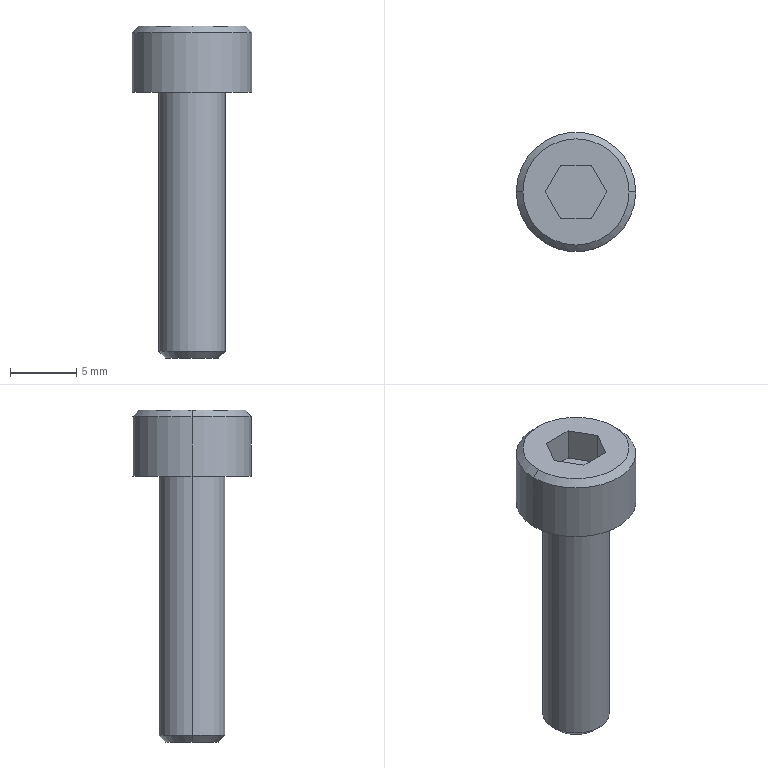Part | STEP file | _GAY01-D20-003_2.stp | 1 solid | 18 faces | box 9 x 9 x 25 mm | volume 670.975 mm3 | plane 10 | cone 4 | cylinder 4 | commonest cylinder face diameters 5 x2 9 x2
STEP:
#1=CARTESIAN_POINT('',(0.,0.,0.));
#2=DIRECTION('',(0.,0.,1.));
#3=DIRECTION('',(1.,0.,0.));
#4=AXIS2_PLACEMENT_3D('',#1,#2,#3);
#5=CARTESIAN_POINT('',(-2.01,0.,-20.));
#6=VERTEX_POINT('',#5);
#7=CARTESIAN_POINT('',(2.01,0.,-20.));
#8=VERTEX_POINT('',#7);
#9=CARTESIAN_POINT('',(0.,0.,-20.));
#10=DIRECTION('',(0.,0.,-1.));
#11=DIRECTION('',(-1.,0.,0.));
#12=AXIS2_PLACEMENT_3D('',#9,#10,#11);
#13=CIRCLE('',#12,2.01);
#14=CARTESIAN_POINT('',(0.,0.,-19.509));
#15=DIRECTION('',(0.,0.,1.));
#16=DIRECTION('',(1.,0.,0.));
#17=AXIS2_PLACEMENT_3D('',#14,#15,#16);
#18=CONICAL_SURFACE('',#17,2.5,0.7854);
#19=CARTESIAN_POINT('',(3.142,-0.4905));
#20=DIRECTION('',(-1.,0.));
#21=VECTOR('',#20,1.);
#22=LINE('',#19,#21);
#23=(GEOMETRIC_REPRESENTATION_CONTEXT(2)PARAMETRIC_REPRESENTATION_CONTEXT()REPRESENTATION_CONTEXT('',''));
#24=DEFINITIONAL_REPRESENTATION('',(#22),#23);
#25=PCURVE('',#18,#24);
#26=CARTESIAN_POINT('',(0.,2.01,-20.));
#27=DIRECTION('',(0.,0.,1.));
#28=DIRECTION('',(1.,0.,0.));
#29=AXIS2_PLACEMENT_3D('',#26,#27,#28);
#30=PLANE('',#29);
#31=CARTESIAN_POINT('',(-2.01,-2.01));
#32=CARTESIAN_POINT('',(-2.01,1.471));
#33=CARTESIAN_POINT('',(1.005,-0.2692));
#34=CARTESIAN_POINT('',(4.019,-2.01));
#35=CARTESIAN_POINT('',(1.005,-3.75));
#36=CARTESIAN_POINT('',(-2.01,-5.49));
#37=CARTESIAN_POINT('',(-2.01,-2.01));
#38=(BOUNDED_CURVE()B_SPLINE_CURVE(2,(#31,#32,#33,#34,#35,#36,#37),.UNSPECIFIED.,.T.,.F.)B_SPLINE_CURVE_WITH_KNOTS((1,2,2,2,2,1),(-2.094,0.,2.094,4.189,6.283,8.378),.UNSPECIFIED.)CURVE()GEOMETRIC_REPRESENTATION_ITEM()RATIONAL_B_SPLINE_CURVE((1.,0.5,1.,0.5,1.,0.5,1.))REPRESENTATION_ITEM(''));
#39=(GEOMETRIC_REPRESENTATION_CONTEXT(2)PARAMETRIC_REPRESENTATION_CONTEXT()REPRESENTATION_CONTEXT('',''));
#40=DEFINITIONAL_REPRESENTATION('',(#38),#39);
#41=PCURVE('',#30,#40);
#42=SURFACE_CURVE('',#13,(#25,#41),.PCURVE_S1.);
#43=EDGE_CURVE('',#6,#8,#42,.T.);
#44=ORIENTED_EDGE('',*,*,#43,.F.);
#45=CARTESIAN_POINT('',(-2.5,0.,-19.509));
#46=VERTEX_POINT('',#45);
#47=CARTESIAN_POINT('',(-2.5,0.,-19.509));
#48=DIRECTION('',(-0.7071,0.,0.7071));
#49=VECTOR('',#48,1.);
#50=LINE('',#47,#49);
#51=CARTESIAN_POINT('',(3.142,0.));
#52=DIRECTION('',(0.,1.));
#53=VECTOR('',#52,1.);
#54=LINE('',#51,#53);
#55=(GEOMETRIC_REPRESENTATION_CONTEXT(2)PARAMETRIC_REPRESENTATION_CONTEXT()REPRESENTATION_CONTEXT('',''));
#56=DEFINITIONAL_REPRESENTATION('',(#54),#55);
#57=PCURVE('',#18,#56);
#58=CARTESIAN_POINT('',(0.,0.,-19.509));
#59=DIRECTION('',(0.,0.,1.));
#60=DIRECTION('',(1.,0.,0.));
#61=AXIS2_PLACEMENT_3D('',#58,#59,#60);
#62=CONICAL_SURFACE('',#61,2.5,0.7854);
#63=CARTESIAN_POINT('',(3.142,0.));
#64=DIRECTION('',(0.,1.));
#65=VECTOR('',#64,1.);
#66=LINE('',#63,#65);
#67=(GEOMETRIC_REPRESENTATION_CONTEXT(2)PARAMETRIC_REPRESENTATION_CONTEXT()REPRESENTATION_CONTEXT('',''));
#68=DEFINITIONAL_REPRESENTATION('',(#66),#67);
#69=PCURVE('',#62,#68);
#70=SURFACE_CURVE('',#50,(#57,#69),.PCURVE_S1.);
#71=EDGE_CURVE('',#6,#46,#70,.T.);
#72=ORIENTED_EDGE('',*,*,#71,.T.);
#73=CARTESIAN_POINT('',(2.5,0.,-19.509));
#74=VERTEX_POINT('',#73);
#75=CARTESIAN_POINT('',(0.,0.,-19.509));
#76=DIRECTION('',(0.,0.,-1.));
#77=DIRECTION('',(-1.,0.,0.));
#78=AXIS2_PLACEMENT_3D('',#75,#76,#77);
#79=CIRCLE('',#78,2.5);
#80=CARTESIAN_POINT('',(3.142,0.));
#81=DIRECTION('',(-1.,0.));
#82=VECTOR('',#81,1.);
#83=LINE('',#80,#82);
#84=(GEOMETRIC_REPRESENTATION_CONTEXT(2)PARAMETRIC_REPRESENTATION_CONTEXT()REPRESENTATION_CONTEXT('',''));
#85=DEFINITIONAL_REPRESENTATION('',(#83),#84);
#86=PCURVE('',#18,#85);
#87=CARTESIAN_POINT('',(0.,0.,-20.));
#88=DIRECTION('',(0.,0.,1.));
#89=DIRECTION('',(-1.,0.,0.));
#90=AXIS2_PLACEMENT_3D('',#87,#88,#89);
#91=CYLINDRICAL_SURFACE('',#90,2.5);
#92=CARTESIAN_POINT('',(6.283,0.4905));
#93=DIRECTION('',(-1.,0.));
#94=VECTOR('',#93,1.);
#95=LINE('',#92,#94);
#96=(GEOMETRIC_REPRESENTATION_CONTEXT(2)PARAMETRIC_REPRESENTATION_CONTEXT()REPRESENTATION_CONTEXT('',''));
#97=DEFINITIONAL_REPRESENTATION('',(#95),#96);
#98=PCURVE('',#91,#97);
#99=SURFACE_CURVE('',#79,(#86,#98),.PCURVE_S1.);
#100=EDGE_CURVE('',#46,#74,#99,.T.);
#101=ORIENTED_EDGE('',*,*,#100,.T.);
#102=CARTESIAN_POINT('',(2.5,0.,-19.509));
#103=DIRECTION('',(0.7071,0.,0.7071));
#104=VECTOR('',#103,1.);
#105=LINE('',#102,#104);
#106=CARTESIAN_POINT('',(0.,0.));
#107=DIRECTION('',(0.,1.));
#108=VECTOR('',#107,1.);
#109=LINE('',#106,#108);
#110=(GEOMETRIC_REPRESENTATION_CONTEXT(2)PARAMETRIC_REPRESENTATION_CONTEXT()REPRESENTATION_CONTEXT('',''));
#111=DEFINITIONAL_REPRESENTATION('',(#109),#110);
#112=PCURVE('',#18,#111);
#113=CARTESIAN_POINT('',(6.283,0.));
#114=DIRECTION('',(0.,1.));
#115=VECTOR('',#114,1.);
#116=LINE('',#113,#115);
#117=(GEOMETRIC_REPRESENTATION_CONTEXT(2)PARAMETRIC_REPRESENTATION_CONTEXT()REPRESENTATION_CONTEXT('',''));
#118=DEFINITIONAL_REPRESENTATION('',(#116),#117);
#119=PCURVE('',#62,#118);
#120=SURFACE_CURVE('',#105,(#112,#119),.PCURVE_S1.);
#121=EDGE_CURVE('',#8,#74,#120,.T.);
#122=ORIENTED_EDGE('',*,*,#121,.F.);
#123=EDGE_LOOP('',(#44,#72,#101,#122));
#124=FACE_BOUND('',#123,.T.);
#125=ADVANCED_FACE('',(#124),#18,.T.);
#126=CARTESIAN_POINT('',(0.,0.,-19.509));
#127=DIRECTION('',(0.,0.,-1.));
#128=DIRECTION('',(-1.,0.,0.));
#129=AXIS2_PLACEMENT_3D('',#126,#127,#128);
#130=CIRCLE('',#129,2.5);
#131=CARTESIAN_POINT('',(0.,0.,-20.));
#132=DIRECTION('',(0.,0.,1.));
#133=DIRECTION('',(-1.,0.,0.));
#134=AXIS2_PLACEMENT_3D('',#131,#132,#133);
#135=CYLINDRICAL_SURFACE('',#134,2.5);
#136=CARTESIAN_POINT('',(6.283,0.4905));
#137=DIRECTION('',(-1.,0.));
#138=VECTOR('',#137,1.);
#139=LINE('',#136,#138);
#140=(GEOMETRIC_REPRESENTATION_CONTEXT(2)PARAMETRIC_REPRESENTATION_CONTEXT()REPRESENTATION_CONTEXT('',''));
#141=DEFINITIONAL_REPRESENTATION('',(#139),#140);
#142=PCURVE('',#135,#141);
#143=CARTESIAN_POINT('',(9.425,0.));
#144=DIRECTION('',(-1.,0.));
#145=VECTOR('',#144,1.);
#146=LINE('',#143,#145);
#147=(GEOMETRIC_REPRESENTATION_CONTEXT(2)PARAMETRIC_REPRESENTATION_CONTEXT()REPRESENTATION_CONTEXT('',''));
#148=DEFINITIONAL_REPRESENTATION('',(#146),#147);
#149=PCURVE('',#62,#148);
#150=SURFACE_CURVE('',#130,(#142,#149),.PCURVE_S1.);
#151=EDGE_CURVE('',#74,#46,#150,.T.);
#152=ORIENTED_EDGE('',*,*,#151,.F.);
#153=CARTESIAN_POINT('',(2.5,0.,0.));
#154=VERTEX_POINT('',#153);
#155=CARTESIAN_POINT('',(2.5,0.,-20.));
#156=DIRECTION('',(0.,0.,1.));
#157=VECTOR('',#156,1.);
#158=LINE('',#155,#157);
#159=CARTESIAN_POINT('',(3.142,0.));
#160=DIRECTION('',(0.,1.));
#161=VECTOR('',#160,1.);
#162=LINE('',#159,#161);
#163=(GEOMETRIC_REPRESENTATION_CONTEXT(2)PARAMETRIC_REPRESENTATION_CONTEXT()REPRESENTATION_CONTEXT('',''));
#164=DEFINITIONAL_REPRESENTATION('',(#162),#163);
#165=PCURVE('',#135,#164);
#166=CARTESIAN_POINT('',(3.142,0.));
#167=DIRECTION('',(0.,1.));
#168=VECTOR('',#167,1.);
#169=LINE('',#166,#168);
#170=(GEOMETRIC_REPRESENTATION_CONTEXT(2)PARAMETRIC_REPRESENTATION_CONTEXT()REPRESENTATION_CONTEXT('',''));
#171=DEFINITIONAL_REPRESENTATION('',(#169),#170);
#172=PCURVE('',#91,#171);
#173=SURFACE_CURVE('',#158,(#165,#172),.PCURVE_S1.);
#174=EDGE_CURVE('',#74,#154,#173,.T.);
#175=ORIENTED_EDGE('',*,*,#174,.T.);
#176=CARTESIAN_POINT('',(-2.5,0.,0.));
#177=VERTEX_POINT('',#176);
#178=CARTESIAN_POINT('',(0.,0.,0.));
#179=DIRECTION('',(0.,0.,-1.));
#180=DIRECTION('',(-1.,0.,0.));
#181=AXIS2_PLACEMENT_3D('',#178,#179,#180);
#182=CIRCLE('',#181,2.5);
#183=CARTESIAN_POINT('',(6.283,20.));
#184=DIRECTION('',(-1.,0.));
#185=VECTOR('',#184,1.);
#186=LINE('',#183,#185);
#187=(GEOMETRIC_REPRESENTATION_CONTEXT(2)PARAMETRIC_REPRESENTATION_CONTEXT()REPRESENTATION_CONTEXT('',''));
#188=DEFINITIONAL_REPRESENTATION('',(#186),#187);
#189=PCURVE('',#135,#188);
#190=CARTESIAN_POINT('',(0.,4.5,0.));
#191=DIRECTION('',(0.,0.,1.));
#192=DIRECTION('',(1.,0.,0.));
#193=AXIS2_PLACEMENT_3D('',#190,#191,#192);
#194=PLANE('',#193);
#195=CARTESIAN_POINT('',(-2.5,-4.5));
#196=CARTESIAN_POINT('',(-2.5,-0.1699));
#197=CARTESIAN_POINT('',(1.25,-2.335));
#198=CARTESIAN_POINT('',(5.,-4.5));
#199=CARTESIAN_POINT('',(1.25,-6.665));
#200=CARTESIAN_POINT('',(-2.5,-8.83));
#201=CARTESIAN_POINT('',(-2.5,-4.5));
#202=(BOUNDED_CURVE()B_SPLINE_CURVE(2,(#195,#196,#197,#198,#199,#200,#201),.UNSPECIFIED.,.T.,.F.)B_SPLINE_CURVE_WITH_KNOTS((1,2,2,2,2,1),(-2.094,0.,2.094,4.189,6.283,8.378),.UNSPECIFIED.)CURVE()GEOMETRIC_REPRESENTATION_ITEM()RATIONAL_B_SPLINE_CURVE((1.,0.5,1.,0.5,1.,0.5,1.))REPRESENTATION_ITEM(''));
#203=(GEOMETRIC_REPRESENTATION_CONTEXT(2)PARAMETRIC_REPRESENTATION_CONTEXT()REPRESENTATION_CONTEXT('',''));
#204=DEFINITIONAL_REPRESENTATION('',(#202),#203);
#205=PCURVE('',#194,#204);
#206=SURFACE_CURVE('',#182,(#189,#205),.PCURVE_S1.);
#207=EDGE_CURVE('',#154,#177,#206,.T.);
#208=ORIENTED_EDGE('',*,*,#207,.T.);
#209=CARTESIAN_POINT('',(-2.5,0.,-20.));
#210=DIRECTION('',(0.,0.,1.));
#211=VECTOR('',#210,1.);
#212=LINE('',#209,#211);
#213=CARTESIAN_POINT('',(0.,0.));
#214=DIRECTION('',(0.,1.));
#215=VECTOR('',#214,1.);
#216=LINE('',#213,#215);
#217=(GEOMETRIC_REPRESENTATION_CONTEXT(2)PARAMETRIC_REPRESENTATION_CONTEXT()REPRESENTATION_CONTEXT('',''));
#218=DEFINITIONAL_REPRESENTATION('',(#216),#217);
#219=PCURVE('',#135,#218);
#220=CARTESIAN_POINT('',(6.283,0.));
#221=DIRECTION('',(0.,1.));
#222=VECTOR('',#221,1.);
#223=LINE('',#220,#222);
#224=(GEOMETRIC_REPRESENTATION_CONTEXT(2)PARAMETRIC_REPRESENTATION_CONTEXT()REPRESENTATION_CONTEXT('',''));
#225=DEFINITIONAL_REPRESENTATION('',(#223),#224);
#226=PCURVE('',#91,#225);
#227=SURFACE_CURVE('',#212,(#219,#226),.PCURVE_S1.);
#228=EDGE_CURVE('',#46,#177,#227,.T.);
#229=ORIENTED_EDGE('',*,*,#228,.F.);
#230=EDGE_LOOP('',(#152,#175,#208,#229));
#231=FACE_BOUND('',#230,.T.);
#232=ADVANCED_FACE('',(#231),#135,.T.);
#233=CARTESIAN_POINT('',(4.5,0.,0.));
#234=VERTEX_POINT('',#233);
#235=CARTESIAN_POINT('',(-4.5,0.,0.));
#236=VERTEX_POINT('',#235);
#237=CARTESIAN_POINT('',(0.,0.,0.));
#238=DIRECTION('',(0.,0.,-1.));
#239=DIRECTION('',(-1.,0.,0.));
#240=AXIS2_PLACEMENT_3D('',#237,#238,#239);
#241=CIRCLE('',#240,4.5);
#242=CARTESIAN_POINT('',(0.,0.,-20.));
#243=DIRECTION('',(0.,0.,1.));
#244=DIRECTION('',(-1.,0.,0.));
#245=AXIS2_PLACEMENT_3D('',#242,#243,#244);
#246=CYLINDRICAL_SURFACE('',#245,4.5);
#247=CARTESIAN_POINT('',(6.283,20.));
#248=DIRECTION('',(-1.,0.));
#249=VECTOR('',#248,1.);
#250=LINE('',#247,#249);
#251=(GEOMETRIC_REPRESENTATION_CONTEXT(2)PARAMETRIC_REPRESENTATION_CONTEXT()REPRESENTATION_CONTEXT('',''));
#252=DEFINITIONAL_REPRESENTATION('',(#250),#251);
#253=PCURVE('',#246,#252);
#254=CARTESIAN_POINT('',(-4.5,-4.5));
#255=CARTESIAN_POINT('',(-4.5,3.294));
#256=CARTESIAN_POINT('',(2.25,-0.6029));
#257=CARTESIAN_POINT('',(9.,-4.5));
#258=CARTESIAN_POINT('',(2.25,-8.397));
#259=CARTESIAN_POINT('',(-4.5,-12.294));
#260=CARTESIAN_POINT('',(-4.5,-4.5));
#261=(BOUNDED_CURVE()B_SPLINE_CURVE(2,(#254,#255,#256,#257,#258,#259,#260),.UNSPECIFIED.,.T.,.F.)B_SPLINE_CURVE_WITH_KNOTS((1,2,2,2,2,1),(-2.094,0.,2.094,4.189,6.283,8.378),.UNSPECIFIED.)CURVE()GEOMETRIC_REPRESENTATION_ITEM()RATIONAL_B_SPLINE_CURVE((1.,0.5,1.,0.5,1.,0.5,1.))REPRESENTATION_ITEM(''));
#262=(GEOMETRIC_REPRESENTATION_CONTEXT(2)PARAMETRIC_REPRESENTATION_CONTEXT()REPRESENTATION_CONTEXT('',''));
#263=DEFINITIONAL_REPRESENTATION('',(#261),#262);
#264=PCURVE('',#194,#263);
#265=SURFACE_CURVE('',#241,(#253,#264),.PCURVE_S1.);
#266=EDGE_CURVE('',#234,#236,#265,.T.);
#267=ORIENTED_EDGE('',*,*,#266,.F.);
#268=CARTESIAN_POINT('',(4.5,0.,4.5));
#269=VERTEX_POINT('',#268);
#270=CARTESIAN_POINT('',(4.5,0.,-20.));
#271=DIRECTION('',(0.,0.,1.));
#272=VECTOR('',#271,1.);
#273=LINE('',#270,#272);
#274=CARTESIAN_POINT('',(3.142,0.));
#275=DIRECTION('',(0.,1.));
#276=VECTOR('',#275,1.);
#277=LINE('',#274,#276);
#278=(GEOMETRIC_REPRESENTATION_CONTEXT(2)PARAMETRIC_REPRESENTATION_CONTEXT()REPRESENTATION_CONTEXT('',''));
#279=DEFINITIONAL_REPRESENTATION('',(#277),#278);
#280=PCURVE('',#246,#279);
#281=CARTESIAN_POINT('',(0.,0.,-20.));
#282=DIRECTION('',(0.,0.,1.));
#283=DIRECTION('',(-1.,0.,0.));
#284=AXIS2_PLACEMENT_3D('',#281,#282,#283);
#285=CYLINDRICAL_SURFACE('',#284,4.5);
#286=CARTESIAN_POINT('',(3.142,0.));
#287=DIRECTION('',(0.,1.));
#288=VECTOR('',#287,1.);
#289=LINE('',#286,#288);
#290=(GEOMETRIC_REPRESENTATION_CONTEXT(2)PARAMETRIC_REPRESENTATION_CONTEXT()REPRESENTATION_CONTEXT('',''));
#291=DEFINITIONAL_REPRESENTATION('',(#289),#290);
#292=PCURVE('',#285,#291);
#293=SURFACE_CURVE('',#273,(#280,#292),.PCURVE_S1.);
#294=EDGE_CURVE('',#234,#269,#293,.T.);
#295=ORIENTED_EDGE('',*,*,#294,.T.);
#296=CARTESIAN_POINT('',(-4.5,0.,4.5));
#297=VERTEX_POINT('',#296);
#298=CARTESIAN_POINT('',(0.,0.,4.5));
#299=DIRECTION('',(0.,0.,-1.));
#300=DIRECTION('',(-1.,0.,0.));
#301=AXIS2_PLACEMENT_3D('',#298,#299,#300);
#302=CIRCLE('',#301,4.5);
#303=CARTESIAN_POINT('',(6.283,24.5));
#304=DIRECTION('',(-1.,0.));
#305=VECTOR('',#304,1.);
#306=LINE('',#303,#305);
#307=(GEOMETRIC_REPRESENTATION_CONTEXT(2)PARAMETRIC_REPRESENTATION_CONTEXT()REPRESENTATION_CONTEXT('',''));
#308=DEFINITIONAL_REPRESENTATION('',(#306),#307);
#309=PCURVE('',#246,#308);
#310=CARTESIAN_POINT('',(0.,0.,5.));
#311=DIRECTION('',(0.,0.,-1.));
#312=DIRECTION('',(-1.,0.,0.));
#313=AXIS2_PLACEMENT_3D('',#310,#311,#312);
#314=CONICAL_SURFACE('',#313,4.,0.7854);
#315=CARTESIAN_POINT('',(0.,0.5));
#316=DIRECTION('',(1.,0.));
#317=VECTOR('',#316,1.);
#318=LINE('',#315,#317);
#319=(GEOMETRIC_REPRESENTATION_CONTEXT(2)PARAMETRIC_REPRESENTATION_CONTEXT()REPRESENTATION_CONTEXT('',''));
#320=DEFINITIONAL_REPRESENTATION('',(#318),#319);
#321=PCURVE('',#314,#320);
#322=SURFACE_CURVE('',#302,(#309,#321),.PCURVE_S1.);
#323=EDGE_CURVE('',#269,#297,#322,.T.);
#324=ORIENTED_EDGE('',*,*,#323,.T.);
#325=CARTESIAN_POINT('',(-4.5,0.,-20.));
#326=DIRECTION('',(0.,0.,1.));
#327=VECTOR('',#326,1.);
#328=LINE('',#325,#327);
#329=CARTESIAN_POINT('',(0.,0.));
#330=DIRECTION('',(0.,1.));
#331=VECTOR('',#330,1.);
#332=LINE('',#329,#331);
#333=(GEOMETRIC_REPRESENTATION_CONTEXT(2)PARAMETRIC_REPRESENTATION_CONTEXT()REPRESENTATION_CONTEXT('',''));
#334=DEFINITIONAL_REPRESENTATION('',(#332),#333);
#335=PCURVE('',#246,#334);
#336=CARTESIAN_POINT('',(6.283,0.));
#337=DIRECTION('',(0.,1.));
#338=VECTOR('',#337,1.);
#339=LINE('',#336,#338);
#340=(GEOMETRIC_REPRESENTATION_CONTEXT(2)PARAMETRIC_REPRESENTATION_CONTEXT()REPRESENTATION_CONTEXT('',''));
#341=DEFINITIONAL_REPRESENTATION('',(#339),#340);
#342=PCURVE('',#285,#341);
#343=SURFACE_CURVE('',#328,(#335,#342),.PCURVE_S1.);
#344=EDGE_CURVE('',#236,#297,#343,.T.);
#345=ORIENTED_EDGE('',*,*,#344,.F.);
#346=EDGE_LOOP('',(#267,#295,#324,#345));
#347=FACE_BOUND('',#346,.T.);
#348=ADVANCED_FACE('',(#347),#246,.T.);
#349=CARTESIAN_POINT('',(-4.,0.,5.));
#350=VERTEX_POINT('',#349);
#351=CARTESIAN_POINT('',(4.,0.,5.));
#352=VERTEX_POINT('',#351);
#353=CARTESIAN_POINT('',(0.,0.,5.));
#354=DIRECTION('',(0.,0.,-1.));
#355=DIRECTION('',(-1.,0.,0.));
#356=AXIS2_PLACEMENT_3D('',#353,#354,#355);
#357=CIRCLE('',#356,4.);
#358=CARTESIAN_POINT('',(0.,0.,5.));
#359=DIRECTION('',(0.,0.,-1.));
#360=DIRECTION('',(-1.,0.,0.));
#361=AXIS2_PLACEMENT_3D('',#358,#359,#360);
#362=CONICAL_SURFACE('',#361,4.,0.7854);
#363=CARTESIAN_POINT('',(0.,0.));
#364=DIRECTION('',(1.,0.));
#365=VECTOR('',#364,1.);
#366=LINE('',#363,#365);
#367=(GEOMETRIC_REPRESENTATION_CONTEXT(2)PARAMETRIC_REPRESENTATION_CONTEXT()REPRESENTATION_CONTEXT('',''));
#368=DEFINITIONAL_REPRESENTATION('',(#366),#367);
#369=PCURVE('',#362,#368);
#370=CARTESIAN_POINT('',(0.,0.,5.));
#371=DIRECTION('',(0.,0.,-1.));
#372=DIRECTION('',(0.,-1.,0.));
#373=AXIS2_PLACEMENT_3D('',#370,#371,#372);
#374=PLANE('',#373);
#375=CARTESIAN_POINT('',(0.,0.));
#376=DIRECTION('',(0.,1.));
#377=AXIS2_PLACEMENT_2D('',#375,#376);
#378=CIRCLE('',#377,4.);
#379=(GEOMETRIC_REPRESENTATION_CONTEXT(2)PARAMETRIC_REPRESENTATION_CONTEXT()REPRESENTATION_CONTEXT('',''));
#380=DEFINITIONAL_REPRESENTATION('',(#378),#379);
#381=PCURVE('',#374,#380);
#382=SURFACE_CURVE('',#357,(#369,#381),.PCURVE_S1.);
#383=EDGE_CURVE('',#350,#352,#382,.T.);
#384=ORIENTED_EDGE('',*,*,#383,.T.);
#385=CARTESIAN_POINT('',(4.,0.,5.));
#386=DIRECTION('',(0.7071,0.,-0.7071));
#387=VECTOR('',#386,1.);
#388=LINE('',#385,#387);
#389=CARTESIAN_POINT('',(3.142,0.));
#390=DIRECTION('',(0.,1.));
#391=VECTOR('',#390,1.);
#392=LINE('',#389,#391);
#393=(GEOMETRIC_REPRESENTATION_CONTEXT(2)PARAMETRIC_REPRESENTATION_CONTEXT()REPRESENTATION_CONTEXT('',''));
#394=DEFINITIONAL_REPRESENTATION('',(#392),#393);
#395=PCURVE('',#362,#394);
#396=CARTESIAN_POINT('',(3.142,0.));
#397=DIRECTION('',(0.,1.));
#398=VECTOR('',#397,1.);
#399=LINE('',#396,#398);
#400=(GEOMETRIC_REPRESENTATION_CONTEXT(2)PARAMETRIC_REPRESENTATION_CONTEXT()REPRESENTATION_CONTEXT('',''));
#401=DEFINITIONAL_REPRESENTATION('',(#399),#400);
#402=PCURVE('',#314,#401);
#403=SURFACE_CURVE('',#388,(#395,#402),.PCURVE_S1.);
#404=EDGE_CURVE('',#352,#269,#403,.T.);
#405=ORIENTED_EDGE('',*,*,#404,.T.);
#406=CARTESIAN_POINT('',(0.,0.,4.5));
#407=DIRECTION('',(0.,0.,-1.));
#408=DIRECTION('',(-1.,0.,0.));
#409=AXIS2_PLACEMENT_3D('',#406,#407,#408);
#410=CIRCLE('',#409,4.5);
#411=CARTESIAN_POINT('',(0.,0.5));
#412=DIRECTION('',(1.,0.));
#413=VECTOR('',#412,1.);
#414=LINE('',#411,#413);
#415=(GEOMETRIC_REPRESENTATION_CONTEXT(2)PARAMETRIC_REPRESENTATION_CONTEXT()REPRESENTATION_CONTEXT('',''));
#416=DEFINITIONAL_REPRESENTATION('',(#414),#415);
#417=PCURVE('',#362,#416);
#418=CARTESIAN_POINT('',(6.283,24.5));
#419=DIRECTION('',(-1.,0.));
#420=VECTOR('',#419,1.);
#421=LINE('',#418,#420);
#422=(GEOMETRIC_REPRESENTATION_CONTEXT(2)PARAMETRIC_REPRESENTATION_CONTEXT()REPRESENTATION_CONTEXT('',''));
#423=DEFINITIONAL_REPRESENTATION('',(#421),#422);
#424=PCURVE('',#285,#423);
#425=SURFACE_CURVE('',#410,(#417,#424),.PCURVE_S1.);
#426=EDGE_CURVE('',#297,#269,#425,.T.);
#427=ORIENTED_EDGE('',*,*,#426,.F.);
#428=CARTESIAN_POINT('',(-4.,0.,5.));
#429=DIRECTION('',(-0.7071,0.,-0.7071));
#430=VECTOR('',#429,1.);
#431=LINE('',#428,#430);
#432=CARTESIAN_POINT('',(0.,0.));
#433=DIRECTION('',(0.,1.));
#434=VECTOR('',#433,1.);
#435=LINE('',#432,#434);
#436=(GEOMETRIC_REPRESENTATION_CONTEXT(2)PARAMETRIC_REPRESENTATION_CONTEXT()REPRESENTATION_CONTEXT('',''));
#437=DEFINITIONAL_REPRESENTATION('',(#435),#436);
#438=PCURVE('',#362,#437);
#439=CARTESIAN_POINT('',(6.283,0.));
#440=DIRECTION('',(0.,1.));
#441=VECTOR('',#440,1.);
#442=LINE('',#439,#441);
#443=(GEOMETRIC_REPRESENTATION_CONTEXT(2)PARAMETRIC_REPRESENTATION_CONTEXT()REPRESENTATION_CONTEXT('',''));
#444=DEFINITIONAL_REPRESENTATION('',(#442),#443);
#445=PCURVE('',#314,#444);
#446=SURFACE_CURVE('',#431,(#438,#445),.PCURVE_S1.);
#447=EDGE_CURVE('',#350,#297,#446,.T.);
#448=ORIENTED_EDGE('',*,*,#447,.F.);
#449=EDGE_LOOP('',(#384,#405,#427,#448));
#450=FACE_BOUND('',#449,.T.);
#451=ADVANCED_FACE('',(#450),#362,.T.);
#452=ORIENTED_EDGE('',*,*,#404,.F.);
#453=CARTESIAN_POINT('',(0.,0.,5.));
#454=DIRECTION('',(0.,0.,-1.));
#455=DIRECTION('',(-1.,0.,0.));
#456=AXIS2_PLACEMENT_3D('',#453,#454,#455);
#457=CIRCLE('',#456,4.);
#458=CARTESIAN_POINT('',(0.,0.));
#459=DIRECTION('',(1.,0.));
#460=VECTOR('',#459,1.);
#461=LINE('',#458,#460);
#462=(GEOMETRIC_REPRESENTATION_CONTEXT(2)PARAMETRIC_REPRESENTATION_CONTEXT()REPRESENTATION_CONTEXT('',''));
#463=DEFINITIONAL_REPRESENTATION('',(#461),#462);
#464=PCURVE('',#314,#463);
#465=CARTESIAN_POINT('',(0.,0.));
#466=DIRECTION('',(0.,1.));
#467=AXIS2_PLACEMENT_2D('',#465,#466);
#468=CIRCLE('',#467,4.);
#469=(GEOMETRIC_REPRESENTATION_CONTEXT(2)PARAMETRIC_REPRESENTATION_CONTEXT()REPRESENTATION_CONTEXT('',''));
#470=DEFINITIONAL_REPRESENTATION('',(#468),#469);
#471=PCURVE('',#374,#470);
#472=SURFACE_CURVE('',#457,(#464,#471),.PCURVE_S1.);
#473=EDGE_CURVE('',#352,#350,#472,.T.);
#474=ORIENTED_EDGE('',*,*,#473,.T.);
#475=ORIENTED_EDGE('',*,*,#447,.T.);
#476=ORIENTED_EDGE('',*,*,#323,.F.);
#477=EDGE_LOOP('',(#452,#474,#475,#476));
#478=FACE_BOUND('',#477,.T.);
#479=ADVANCED_FACE('',(#478),#314,.T.);
#480=ORIENTED_EDGE('',*,*,#294,.F.);
#481=CARTESIAN_POINT('',(0.,0.,0.));
#482=DIRECTION('',(0.,0.,-1.));
#483=DIRECTION('',(-1.,0.,0.));
#484=AXIS2_PLACEMENT_3D('',#481,#482,#483);
#485=CIRCLE('',#484,4.5);
#486=CARTESIAN_POINT('',(6.283,20.));
#487=DIRECTION('',(-1.,0.));
#488=VECTOR('',#487,1.);
#489=LINE('',#486,#488);
#490=(GEOMETRIC_REPRESENTATION_CONTEXT(2)PARAMETRIC_REPRESENTATION_CONTEXT()REPRESENTATION_CONTEXT('',''));
#491=DEFINITIONAL_REPRESENTATION('',(#489),#490);
#492=PCURVE('',#285,#491);
#493=CARTESIAN_POINT('',(-4.5,-4.5));
#494=CARTESIAN_POINT('',(-4.5,3.294));
#495=CARTESIAN_POINT('',(2.25,-0.6029));
#496=CARTESIAN_POINT('',(9.,-4.5));
#497=CARTESIAN_POINT('',(2.25,-8.397));
#498=CARTESIAN_POINT('',(-4.5,-12.294));
#499=CARTESIAN_POINT('',(-4.5,-4.5));
#500=(BOUNDED_CURVE()B_SPLINE_CURVE(2,(#493,#494,#495,#496,#497,#498,#499),.UNSPECIFIED.,.T.,.F.)B_SPLINE_CURVE_WITH_KNOTS((1,2,2,2,2,1),(-2.094,0.,2.094,4.189,6.283,8.378),.UNSPECIFIED.)CURVE()GEOMETRIC_REPRESENTATION_ITEM()RATIONAL_B_SPLINE_CURVE((1.,0.5,1.,0.5,1.,0.5,1.))REPRESENTATION_ITEM(''));
#501=(GEOMETRIC_REPRESENTATION_CONTEXT(2)PARAMETRIC_REPRESENTATION_CONTEXT()REPRESENTATION_CONTEXT('',''));
#502=DEFINITIONAL_REPRESENTATION('',(#500),#501);
#503=PCURVE('',#194,#502);
#504=SURFACE_CURVE('',#485,(#492,#503),.PCURVE_S1.);
#505=EDGE_CURVE('',#236,#234,#504,.T.);
#506=ORIENTED_EDGE('',*,*,#505,.F.);
#507=ORIENTED_EDGE('',*,*,#344,.T.);
#508=ORIENTED_EDGE('',*,*,#426,.T.);
#509=EDGE_LOOP('',(#480,#506,#507,#508));
#510=FACE_BOUND('',#509,.T.);
#511=ADVANCED_FACE('',(#510),#285,.T.);
#512=CARTESIAN_POINT('',(0.,0.,0.));
#513=DIRECTION('',(0.,0.,-1.));
#514=DIRECTION('',(-1.,0.,0.));
#515=AXIS2_PLACEMENT_3D('',#512,#513,#514);
#516=CIRCLE('',#515,2.5);
#517=CARTESIAN_POINT('',(-2.5,-4.5));
#518=CARTESIAN_POINT('',(-2.5,-0.1699));
#519=CARTESIAN_POINT('',(1.25,-2.335));
#520=CARTESIAN_POINT('',(5.,-4.5));
#521=CARTESIAN_POINT('',(1.25,-6.665));
#522=CARTESIAN_POINT('',(-2.5,-8.83));
#523=CARTESIAN_POINT('',(-2.5,-4.5));
#524=(BOUNDED_CURVE()B_SPLINE_CURVE(2,(#517,#518,#519,#520,#521,#522,#523),.UNSPECIFIED.,.T.,.F.)B_SPLINE_CURVE_WITH_KNOTS((1,2,2,2,2,1),(-2.094,0.,2.094,4.189,6.283,8.378),.UNSPECIFIED.)CURVE()GEOMETRIC_REPRESENTATION_ITEM()RATIONAL_B_SPLINE_CURVE((1.,0.5,1.,0.5,1.,0.5,1.))REPRESENTATION_ITEM(''));
#525=(GEOMETRIC_REPRESENTATION_CONTEXT(2)PARAMETRIC_REPRESENTATION_CONTEXT()REPRESENTATION_CONTEXT('',''));
#526=DEFINITIONAL_REPRESENTATION('',(#524),#525);
#527=PCURVE('',#194,#526);
#528=CARTESIAN_POINT('',(6.283,20.));
#529=DIRECTION('',(-1.,0.));
#530=VECTOR('',#529,1.);
#531=LINE('',#528,#530);
#532=(GEOMETRIC_REPRESENTATION_CONTEXT(2)PARAMETRIC_REPRESENTATION_CONTEXT()REPRESENTATION_CONTEXT('',''));
#533=DEFINITIONAL_REPRESENTATION('',(#531),#532);
#534=PCURVE('',#91,#533);
#535=SURFACE_CURVE('',#516,(#527,#534),.PCURVE_S1.);
#536=EDGE_CURVE('',#177,#154,#535,.T.);
#537=ORIENTED_EDGE('',*,*,#536,.F.);
#538=ORIENTED_EDGE('',*,*,#207,.F.);
#539=EDGE_LOOP('',(#537,#538));
#540=FACE_BOUND('',#539,.T.);
#541=ORIENTED_EDGE('',*,*,#505,.T.);
#542=ORIENTED_EDGE('',*,*,#266,.T.);
#543=EDGE_LOOP('',(#541,#542));
#544=FACE_BOUND('',#543,.T.);
#545=ADVANCED_FACE('',(#540,#544),#194,.F.);
#546=ORIENTED_EDGE('',*,*,#174,.F.);
#547=ORIENTED_EDGE('',*,*,#100,.F.);
#548=ORIENTED_EDGE('',*,*,#228,.T.);
#549=ORIENTED_EDGE('',*,*,#536,.T.);
#550=EDGE_LOOP('',(#546,#547,#548,#549));
#551=FACE_BOUND('',#550,.T.);
#552=ADVANCED_FACE('',(#551),#91,.T.);
#553=ORIENTED_EDGE('',*,*,#71,.F.);
#554=CARTESIAN_POINT('',(0.,0.,-20.));
#555=DIRECTION('',(0.,0.,-1.));
#556=DIRECTION('',(-1.,0.,0.));
#557=AXIS2_PLACEMENT_3D('',#554,#555,#556);
#558=CIRCLE('',#557,2.01);
#559=CARTESIAN_POINT('',(9.425,-0.4905));
#560=DIRECTION('',(-1.,0.));
#561=VECTOR('',#560,1.);
#562=LINE('',#559,#561);
#563=(GEOMETRIC_REPRESENTATION_CONTEXT(2)PARAMETRIC_REPRESENTATION_CONTEXT()REPRESENTATION_CONTEXT('',''));
#564=DEFINITIONAL_REPRESENTATION('',(#562),#563);
#565=PCURVE('',#62,#564);
#566=CARTESIAN_POINT('',(-2.01,-2.01));
#567=CARTESIAN_POINT('',(-2.01,1.471));
#568=CARTESIAN_POINT('',(1.005,-0.2692));
#569=CARTESIAN_POINT('',(4.019,-2.01));
#570=CARTESIAN_POINT('',(1.005,-3.75));
#571=CARTESIAN_POINT('',(-2.01,-5.49));
#572=CARTESIAN_POINT('',(-2.01,-2.01));
#573=(BOUNDED_CURVE()B_SPLINE_CURVE(2,(#566,#567,#568,#569,#570,#571,#572),.UNSPECIFIED.,.T.,.F.)B_SPLINE_CURVE_WITH_KNOTS((1,2,2,2,2,1),(-2.094,0.,2.094,4.189,6.283,8.378),.UNSPECIFIED.)CURVE()GEOMETRIC_REPRESENTATION_ITEM()RATIONAL_B_SPLINE_CURVE((1.,0.5,1.,0.5,1.,0.5,1.))REPRESENTATION_ITEM(''));
#574=(GEOMETRIC_REPRESENTATION_CONTEXT(2)PARAMETRIC_REPRESENTATION_CONTEXT()REPRESENTATION_CONTEXT('',''));
#575=DEFINITIONAL_REPRESENTATION('',(#573),#574);
#576=PCURVE('',#30,#575);
#577=SURFACE_CURVE('',#558,(#565,#576),.PCURVE_S1.);
#578=EDGE_CURVE('',#8,#6,#577,.T.);
#579=ORIENTED_EDGE('',*,*,#578,.F.);
#580=ORIENTED_EDGE('',*,*,#121,.T.);
#581=ORIENTED_EDGE('',*,*,#151,.T.);
#582=EDGE_LOOP('',(#553,#579,#580,#581));
#583=FACE_BOUND('',#582,.T.);
#584=ADVANCED_FACE('',(#583),#62,.T.);
#585=ORIENTED_EDGE('',*,*,#578,.T.);
#586=ORIENTED_EDGE('',*,*,#43,.T.);
#587=EDGE_LOOP('',(#585,#586));
#588=FACE_BOUND('',#587,.T.);
#589=ADVANCED_FACE('',(#588),#30,.F.);
#590=CARTESIAN_POINT('',(-1.155,-2.,5.));
#591=VERTEX_POINT('',#590);
#592=CARTESIAN_POINT('',(1.155,-2.,5.));
#593=VERTEX_POINT('',#592);
#594=CARTESIAN_POINT('',(-1.155,-2.,5.));
#595=DIRECTION('',(1.,0.,0.));
#596=VECTOR('',#595,1.);
#597=LINE('',#594,#596);
#598=CARTESIAN_POINT('',(-1.155,-2.,2.5));
#599=DIRECTION('',(0.,-1.,0.));
#600=DIRECTION('',(0.,0.,-1.));
#601=AXIS2_PLACEMENT_3D('',#598,#599,#600);
#602=PLANE('',#601);
#603=CARTESIAN_POINT('',(-2.5,0.));
#604=DIRECTION('',(0.,1.));
#605=VECTOR('',#604,1.);
#606=LINE('',#603,#605);
#607=(GEOMETRIC_REPRESENTATION_CONTEXT(2)PARAMETRIC_REPRESENTATION_CONTEXT()REPRESENTATION_CONTEXT('',''));
#608=DEFINITIONAL_REPRESENTATION('',(#606),#607);
#609=PCURVE('',#602,#608);
#610=CARTESIAN_POINT('',(2.,1.155));
#611=DIRECTION('',(0.,-1.));
#612=VECTOR('',#611,1.);
#613=LINE('',#610,#612);
#614=(GEOMETRIC_REPRESENTATION_CONTEXT(2)PARAMETRIC_REPRESENTATION_CONTEXT()REPRESENTATION_CONTEXT('',''));
#615=DEFINITIONAL_REPRESENTATION('',(#613),#614);
#616=PCURVE('',#374,#615);
#617=SURFACE_CURVE('',#597,(#609,#616),.PCURVE_S1.);
#618=EDGE_CURVE('',#591,#593,#617,.T.);
#619=ORIENTED_EDGE('',*,*,#618,.T.);
#620=CARTESIAN_POINT('',(1.155,-2.,2.5));
#621=VERTEX_POINT('',#620);
#622=CARTESIAN_POINT('',(1.155,-2.,2.5));
#623=DIRECTION('',(0.,0.,1.));
#624=VECTOR('',#623,1.);
#625=LINE('',#622,#624);
#626=CARTESIAN_POINT('',(0.,2.309));
#627=DIRECTION('',(-1.,0.));
#628=VECTOR('',#627,1.);
#629=LINE('',#626,#628);
#630=(GEOMETRIC_REPRESENTATION_CONTEXT(2)PARAMETRIC_REPRESENTATION_CONTEXT()REPRESENTATION_CONTEXT('',''));
#631=DEFINITIONAL_REPRESENTATION('',(#629),#630);
#632=PCURVE('',#602,#631);
#633=CARTESIAN_POINT('',(1.155,-2.,2.5));
#634=DIRECTION('',(0.866,-0.5,0.));
#635=DIRECTION('',(0.,0.,-1.));
#636=AXIS2_PLACEMENT_3D('',#633,#634,#635);
#637=PLANE('',#636);
#638=CARTESIAN_POINT('',(0.,0.));
#639=DIRECTION('',(-1.,0.));
#640=VECTOR('',#639,1.);
#641=LINE('',#638,#640);
#642=(GEOMETRIC_REPRESENTATION_CONTEXT(2)PARAMETRIC_REPRESENTATION_CONTEXT()REPRESENTATION_CONTEXT('',''));
#643=DEFINITIONAL_REPRESENTATION('',(#641),#642);
#644=PCURVE('',#637,#643);
#645=SURFACE_CURVE('',#625,(#632,#644),.PCURVE_S1.);
#646=EDGE_CURVE('',#621,#593,#645,.T.);
#647=ORIENTED_EDGE('',*,*,#646,.F.);
#648=CARTESIAN_POINT('',(-1.155,-2.,2.5));
#649=VERTEX_POINT('',#648);
#650=CARTESIAN_POINT('',(-1.155,-2.,2.5));
#651=DIRECTION('',(1.,0.,0.));
#652=VECTOR('',#651,1.);
#653=LINE('',#650,#652);
#654=CARTESIAN_POINT('',(0.,0.));
#655=DIRECTION('',(0.,1.));
#656=VECTOR('',#655,1.);
#657=LINE('',#654,#656);
#658=(GEOMETRIC_REPRESENTATION_CONTEXT(2)PARAMETRIC_REPRESENTATION_CONTEXT()REPRESENTATION_CONTEXT('',''));
#659=DEFINITIONAL_REPRESENTATION('',(#657),#658);
#660=PCURVE('',#602,#659);
#661=CARTESIAN_POINT('',(0.,0.,2.5));
#662=DIRECTION('',(0.,0.,1.));
#663=DIRECTION('',(1.,0.,0.));
#664=AXIS2_PLACEMENT_3D('',#661,#662,#663);
#665=PLANE('',#664);
#666=CARTESIAN_POINT('',(-1.155,-2.));
#667=DIRECTION('',(1.,0.));
#668=VECTOR('',#667,1.);
#669=LINE('',#666,#668);
#670=(GEOMETRIC_REPRESENTATION_CONTEXT(2)PARAMETRIC_REPRESENTATION_CONTEXT()REPRESENTATION_CONTEXT('',''));
#671=DEFINITIONAL_REPRESENTATION('',(#669),#670);
#672=PCURVE('',#665,#671);
#673=SURFACE_CURVE('',#653,(#660,#672),.PCURVE_S1.);
#674=EDGE_CURVE('',#649,#621,#673,.T.);
#675=ORIENTED_EDGE('',*,*,#674,.F.);
#676=CARTESIAN_POINT('',(-1.155,-2.,2.5));
#677=DIRECTION('',(0.,0.,1.));
#678=VECTOR('',#677,1.);
#679=LINE('',#676,#678);
#680=CARTESIAN_POINT('',(0.,0.));
#681=DIRECTION('',(-1.,0.));
#682=VECTOR('',#681,1.);
#683=LINE('',#680,#682);
#684=(GEOMETRIC_REPRESENTATION_CONTEXT(2)PARAMETRIC_REPRESENTATION_CONTEXT()REPRESENTATION_CONTEXT('',''));
#685=DEFINITIONAL_REPRESENTATION('',(#683),#684);
#686=PCURVE('',#602,#685);
#687=CARTESIAN_POINT('',(-2.309,0.,2.5));
#688=DIRECTION('',(-0.866,-0.5,0.));
#689=DIRECTION('',(-0.5,0.866,0.));
#690=AXIS2_PLACEMENT_3D('',#687,#688,#689);
#691=PLANE('',#690);
#692=CARTESIAN_POINT('',(-2.309,0.));
#693=DIRECTION('',(0.,-1.));
#694=VECTOR('',#693,1.);
#695=LINE('',#692,#694);
#696=(GEOMETRIC_REPRESENTATION_CONTEXT(2)PARAMETRIC_REPRESENTATION_CONTEXT()REPRESENTATION_CONTEXT('',''));
#697=DEFINITIONAL_REPRESENTATION('',(#695),#696);
#698=PCURVE('',#691,#697);
#699=SURFACE_CURVE('',#679,(#686,#698),.PCURVE_S1.);
#700=EDGE_CURVE('',#649,#591,#699,.T.);
#701=ORIENTED_EDGE('',*,*,#700,.T.);
#702=EDGE_LOOP('',(#619,#647,#675,#701));
#703=FACE_BOUND('',#702,.T.);
#704=ADVANCED_FACE('',(#703),#602,.F.);
#705=CARTESIAN_POINT('',(2.309,0.,5.));
#706=VERTEX_POINT('',#705);
#707=CARTESIAN_POINT('',(1.155,-2.,5.));
#708=DIRECTION('',(0.5,0.866,0.));
#709=VECTOR('',#708,1.);
#710=LINE('',#707,#709);
#711=CARTESIAN_POINT('',(-2.5,0.));
#712=DIRECTION('',(0.,1.));
#713=VECTOR('',#712,1.);
#714=LINE('',#711,#713);
#715=(GEOMETRIC_REPRESENTATION_CONTEXT(2)PARAMETRIC_REPRESENTATION_CONTEXT()REPRESENTATION_CONTEXT('',''));
#716=DEFINITIONAL_REPRESENTATION('',(#714),#715);
#717=PCURVE('',#637,#716);
#718=CARTESIAN_POINT('',(2.,-1.155));
#719=DIRECTION('',(-0.866,-0.5));
#720=VECTOR('',#719,1.);
#721=LINE('',#718,#720);
#722=(GEOMETRIC_REPRESENTATION_CONTEXT(2)PARAMETRIC_REPRESENTATION_CONTEXT()REPRESENTATION_CONTEXT('',''));
#723=DEFINITIONAL_REPRESENTATION('',(#721),#722);
#724=PCURVE('',#374,#723);
#725=SURFACE_CURVE('',#710,(#717,#724),.PCURVE_S1.);
#726=EDGE_CURVE('',#593,#706,#725,.T.);
#727=ORIENTED_EDGE('',*,*,#726,.T.);
#728=CARTESIAN_POINT('',(2.309,0.,2.5));
#729=VERTEX_POINT('',#728);
#730=CARTESIAN_POINT('',(2.309,0.,2.5));
#731=DIRECTION('',(0.,0.,1.));
#732=VECTOR('',#731,1.);
#733=LINE('',#730,#732);
#734=CARTESIAN_POINT('',(0.,2.309));
#735=DIRECTION('',(-1.,0.));
#736=VECTOR('',#735,1.);
#737=LINE('',#734,#736);
#738=(GEOMETRIC_REPRESENTATION_CONTEXT(2)PARAMETRIC_REPRESENTATION_CONTEXT()REPRESENTATION_CONTEXT('',''));
#739=DEFINITIONAL_REPRESENTATION('',(#737),#738);
#740=PCURVE('',#637,#739);
#741=CARTESIAN_POINT('',(2.309,0.,2.5));
#742=DIRECTION('',(0.866,0.5,0.));
#743=DIRECTION('',(0.,0.,-1.));
#744=AXIS2_PLACEMENT_3D('',#741,#742,#743);
#745=PLANE('',#744);
#746=CARTESIAN_POINT('',(0.,0.));
#747=DIRECTION('',(-1.,0.));
#748=VECTOR('',#747,1.);
#749=LINE('',#746,#748);
#750=(GEOMETRIC_REPRESENTATION_CONTEXT(2)PARAMETRIC_REPRESENTATION_CONTEXT()REPRESENTATION_CONTEXT('',''));
#751=DEFINITIONAL_REPRESENTATION('',(#749),#750);
#752=PCURVE('',#745,#751);
#753=SURFACE_CURVE('',#733,(#740,#752),.PCURVE_S1.);
#754=EDGE_CURVE('',#729,#706,#753,.T.);
#755=ORIENTED_EDGE('',*,*,#754,.F.);
#756=CARTESIAN_POINT('',(1.155,-2.,2.5));
#757=DIRECTION('',(0.5,0.866,0.));
#758=VECTOR('',#757,1.);
#759=LINE('',#756,#758);
#760=CARTESIAN_POINT('',(0.,0.));
#761=DIRECTION('',(0.,1.));
#762=VECTOR('',#761,1.);
#763=LINE('',#760,#762);
#764=(GEOMETRIC_REPRESENTATION_CONTEXT(2)PARAMETRIC_REPRESENTATION_CONTEXT()REPRESENTATION_CONTEXT('',''));
#765=DEFINITIONAL_REPRESENTATION('',(#763),#764);
#766=PCURVE('',#637,#765);
#767=CARTESIAN_POINT('',(1.155,-2.));
#768=DIRECTION('',(0.5,0.866));
#769=VECTOR('',#768,1.);
#770=LINE('',#767,#769);
#771=(GEOMETRIC_REPRESENTATION_CONTEXT(2)PARAMETRIC_REPRESENTATION_CONTEXT()REPRESENTATION_CONTEXT('',''));
#772=DEFINITIONAL_REPRESENTATION('',(#770),#771);
#773=PCURVE('',#665,#772);
#774=SURFACE_CURVE('',#759,(#766,#773),.PCURVE_S1.);
#775=EDGE_CURVE('',#621,#729,#774,.T.);
#776=ORIENTED_EDGE('',*,*,#775,.F.);
#777=ORIENTED_EDGE('',*,*,#646,.T.);
#778=EDGE_LOOP('',(#727,#755,#776,#777));
#779=FACE_BOUND('',#778,.T.);
#780=ADVANCED_FACE('',(#779),#637,.F.);
#781=CARTESIAN_POINT('',(1.155,2.,5.));
#782=VERTEX_POINT('',#781);
#783=CARTESIAN_POINT('',(2.309,0.,5.));
#784=DIRECTION('',(-0.5,0.866,0.));
#785=VECTOR('',#784,1.);
#786=LINE('',#783,#785);
#787=CARTESIAN_POINT('',(-2.5,0.));
#788=DIRECTION('',(0.,1.));
#789=VECTOR('',#788,1.);
#790=LINE('',#787,#789);
#791=(GEOMETRIC_REPRESENTATION_CONTEXT(2)PARAMETRIC_REPRESENTATION_CONTEXT()REPRESENTATION_CONTEXT('',''));
#792=DEFINITIONAL_REPRESENTATION('',(#790),#791);
#793=PCURVE('',#745,#792);
#794=CARTESIAN_POINT('',(0.,-2.309));
#795=DIRECTION('',(-0.866,0.5));
#796=VECTOR('',#795,1.);
#797=LINE('',#794,#796);
#798=(GEOMETRIC_REPRESENTATION_CONTEXT(2)PARAMETRIC_REPRESENTATION_CONTEXT()REPRESENTATION_CONTEXT('',''));
#799=DEFINITIONAL_REPRESENTATION('',(#797),#798);
#800=PCURVE('',#374,#799);
#801=SURFACE_CURVE('',#786,(#793,#800),.PCURVE_S1.);
#802=EDGE_CURVE('',#706,#782,#801,.T.);
#803=ORIENTED_EDGE('',*,*,#802,.T.);
#804=CARTESIAN_POINT('',(1.155,2.,2.5));
#805=VERTEX_POINT('',#804);
#806=CARTESIAN_POINT('',(1.155,2.,2.5));
#807=DIRECTION('',(0.,0.,1.));
#808=VECTOR('',#807,1.);
#809=LINE('',#806,#808);
#810=CARTESIAN_POINT('',(0.,2.309));
#811=DIRECTION('',(-1.,0.));
#812=VECTOR('',#811,1.);
#813=LINE('',#810,#812);
#814=(GEOMETRIC_REPRESENTATION_CONTEXT(2)PARAMETRIC_REPRESENTATION_CONTEXT()REPRESENTATION_CONTEXT('',''));
#815=DEFINITIONAL_REPRESENTATION('',(#813),#814);
#816=PCURVE('',#745,#815);
#817=CARTESIAN_POINT('',(1.155,2.,2.5));
#818=DIRECTION('',(0.,1.,0.));
#819=DIRECTION('',(1.,0.,0.));
#820=AXIS2_PLACEMENT_3D('',#817,#818,#819);
#821=PLANE('',#820);
#822=CARTESIAN_POINT('',(0.,0.));
#823=DIRECTION('',(0.,-1.));
#824=VECTOR('',#823,1.);
#825=LINE('',#822,#824);
#826=(GEOMETRIC_REPRESENTATION_CONTEXT(2)PARAMETRIC_REPRESENTATION_CONTEXT()REPRESENTATION_CONTEXT('',''));
#827=DEFINITIONAL_REPRESENTATION('',(#825),#826);
#828=PCURVE('',#821,#827);
#829=SURFACE_CURVE('',#809,(#816,#828),.PCURVE_S1.);
#830=EDGE_CURVE('',#805,#782,#829,.T.);
#831=ORIENTED_EDGE('',*,*,#830,.F.);
#832=CARTESIAN_POINT('',(2.309,0.,2.5));
#833=DIRECTION('',(-0.5,0.866,0.));
#834=VECTOR('',#833,1.);
#835=LINE('',#832,#834);
#836=CARTESIAN_POINT('',(0.,0.));
#837=DIRECTION('',(0.,1.));
#838=VECTOR('',#837,1.);
#839=LINE('',#836,#838);
#840=(GEOMETRIC_REPRESENTATION_CONTEXT(2)PARAMETRIC_REPRESENTATION_CONTEXT()REPRESENTATION_CONTEXT('',''));
#841=DEFINITIONAL_REPRESENTATION('',(#839),#840);
#842=PCURVE('',#745,#841);
#843=CARTESIAN_POINT('',(2.309,0.));
#844=DIRECTION('',(-0.5,0.866));
#845=VECTOR('',#844,1.);
#846=LINE('',#843,#845);
#847=(GEOMETRIC_REPRESENTATION_CONTEXT(2)PARAMETRIC_REPRESENTATION_CONTEXT()REPRESENTATION_CONTEXT('',''));
#848=DEFINITIONAL_REPRESENTATION('',(#846),#847);
#849=PCURVE('',#665,#848);
#850=SURFACE_CURVE('',#835,(#842,#849),.PCURVE_S1.);
#851=EDGE_CURVE('',#729,#805,#850,.T.);
#852=ORIENTED_EDGE('',*,*,#851,.F.);
#853=ORIENTED_EDGE('',*,*,#754,.T.);
#854=EDGE_LOOP('',(#803,#831,#852,#853));
#855=FACE_BOUND('',#854,.T.);
#856=ADVANCED_FACE('',(#855),#745,.F.);
#857=ORIENTED_EDGE('',*,*,#830,.T.);
#858=CARTESIAN_POINT('',(-1.155,2.,5.));
#859=VERTEX_POINT('',#858);
#860=CARTESIAN_POINT('',(0.,2.,5.));
#861=DIRECTION('',(1.,0.,0.));
#862=VECTOR('',#861,1.);
#863=LINE('',#860,#862);
#864=CARTESIAN_POINT('',(-1.155,-2.5));
#865=DIRECTION('',(1.,0.));
#866=VECTOR('',#865,1.);
#867=LINE('',#864,#866);
#868=(GEOMETRIC_REPRESENTATION_CONTEXT(2)PARAMETRIC_REPRESENTATION_CONTEXT()REPRESENTATION_CONTEXT('',''));
#869=DEFINITIONAL_REPRESENTATION('',(#867),#868);
#870=PCURVE('',#821,#869);
#871=CARTESIAN_POINT('',(-2.,0.));
#872=DIRECTION('',(0.,-1.));
#873=VECTOR('',#872,1.);
#874=LINE('',#871,#873);
#875=(GEOMETRIC_REPRESENTATION_CONTEXT(2)PARAMETRIC_REPRESENTATION_CONTEXT()REPRESENTATION_CONTEXT('',''));
#876=DEFINITIONAL_REPRESENTATION('',(#874),#875);
#877=PCURVE('',#374,#876);
#878=SURFACE_CURVE('',#863,(#870,#877),.PCURVE_S1.);
#879=EDGE_CURVE('',#859,#782,#878,.T.);
#880=ORIENTED_EDGE('',*,*,#879,.F.);
#881=CARTESIAN_POINT('',(-1.155,2.,2.5));
#882=VERTEX_POINT('',#881);
#883=CARTESIAN_POINT('',(-1.155,2.,2.5));
#884=DIRECTION('',(0.,0.,1.));
#885=VECTOR('',#884,1.);
#886=LINE('',#883,#885);
#887=CARTESIAN_POINT('',(-2.309,0.));
#888=DIRECTION('',(0.,-1.));
#889=VECTOR('',#888,1.);
#890=LINE('',#887,#889);
#891=(GEOMETRIC_REPRESENTATION_CONTEXT(2)PARAMETRIC_REPRESENTATION_CONTEXT()REPRESENTATION_CONTEXT('',''));
#892=DEFINITIONAL_REPRESENTATION('',(#890),#891);
#893=PCURVE('',#821,#892);
#894=CARTESIAN_POINT('',(-1.155,2.,2.5));
#895=DIRECTION('',(-0.866,0.5,0.));
#896=DIRECTION('',(0.,0.,1.));
#897=AXIS2_PLACEMENT_3D('',#894,#895,#896);
#898=PLANE('',#897);
#899=CARTESIAN_POINT('',(0.,0.));
#900=DIRECTION('',(1.,0.));
#901=VECTOR('',#900,1.);
#902=LINE('',#899,#901);
#903=(GEOMETRIC_REPRESENTATION_CONTEXT(2)PARAMETRIC_REPRESENTATION_CONTEXT()REPRESENTATION_CONTEXT('',''));
#904=DEFINITIONAL_REPRESENTATION('',(#902),#903);
#905=PCURVE('',#898,#904);
#906=SURFACE_CURVE('',#886,(#893,#905),.PCURVE_S1.);
#907=EDGE_CURVE('',#882,#859,#906,.T.);
#908=ORIENTED_EDGE('',*,*,#907,.F.);
#909=CARTESIAN_POINT('',(1.155,2.,2.5));
#910=DIRECTION('',(-1.,0.,0.));
#911=VECTOR('',#910,1.);
#912=LINE('',#909,#911);
#913=CARTESIAN_POINT('',(0.,0.));
#914=DIRECTION('',(-1.,0.));
#915=VECTOR('',#914,1.);
#916=LINE('',#913,#915);
#917=(GEOMETRIC_REPRESENTATION_CONTEXT(2)PARAMETRIC_REPRESENTATION_CONTEXT()REPRESENTATION_CONTEXT('',''));
#918=DEFINITIONAL_REPRESENTATION('',(#916),#917);
#919=PCURVE('',#821,#918);
#920=CARTESIAN_POINT('',(1.155,2.));
#921=DIRECTION('',(-1.,0.));
#922=VECTOR('',#921,1.);
#923=LINE('',#920,#922);
#924=(GEOMETRIC_REPRESENTATION_CONTEXT(2)PARAMETRIC_REPRESENTATION_CONTEXT()REPRESENTATION_CONTEXT('',''));
#925=DEFINITIONAL_REPRESENTATION('',(#923),#924);
#926=PCURVE('',#665,#925);
#927=SURFACE_CURVE('',#912,(#919,#926),.PCURVE_S1.);
#928=EDGE_CURVE('',#805,#882,#927,.T.);
#929=ORIENTED_EDGE('',*,*,#928,.F.);
#930=EDGE_LOOP('',(#857,#880,#908,#929));
#931=FACE_BOUND('',#930,.T.);
#932=ADVANCED_FACE('',(#931),#821,.F.);
#933=CARTESIAN_POINT('',(-2.309,0.,5.));
#934=VERTEX_POINT('',#933);
#935=CARTESIAN_POINT('',(-1.155,2.,5.));
#936=DIRECTION('',(-0.5,-0.866,0.));
#937=VECTOR('',#936,1.);
#938=LINE('',#935,#937);
#939=CARTESIAN_POINT('',(2.5,0.));
#940=DIRECTION('',(0.,-1.));
#941=VECTOR('',#940,1.);
#942=LINE('',#939,#941);
#943=(GEOMETRIC_REPRESENTATION_CONTEXT(2)PARAMETRIC_REPRESENTATION_CONTEXT()REPRESENTATION_CONTEXT('',''));
#944=DEFINITIONAL_REPRESENTATION('',(#942),#943);
#945=PCURVE('',#898,#944);
#946=CARTESIAN_POINT('',(-2.,1.155));
#947=DIRECTION('',(0.866,0.5));
#948=VECTOR('',#947,1.);
#949=LINE('',#946,#948);
#950=(GEOMETRIC_REPRESENTATION_CONTEXT(2)PARAMETRIC_REPRESENTATION_CONTEXT()REPRESENTATION_CONTEXT('',''));
#951=DEFINITIONAL_REPRESENTATION('',(#949),#950);
#952=PCURVE('',#374,#951);
#953=SURFACE_CURVE('',#938,(#945,#952),.PCURVE_S1.);
#954=EDGE_CURVE('',#859,#934,#953,.T.);
#955=ORIENTED_EDGE('',*,*,#954,.T.);
#956=CARTESIAN_POINT('',(-2.309,0.,2.5));
#957=VERTEX_POINT('',#956);
#958=CARTESIAN_POINT('',(-2.309,0.,2.5));
#959=DIRECTION('',(0.,0.,1.));
#960=VECTOR('',#959,1.);
#961=LINE('',#958,#960);
#962=CARTESIAN_POINT('',(0.,-2.309));
#963=DIRECTION('',(1.,0.));
#964=VECTOR('',#963,1.);
#965=LINE('',#962,#964);
#966=(GEOMETRIC_REPRESENTATION_CONTEXT(2)PARAMETRIC_REPRESENTATION_CONTEXT()REPRESENTATION_CONTEXT('',''));
#967=DEFINITIONAL_REPRESENTATION('',(#965),#966);
#968=PCURVE('',#898,#967);
#969=CARTESIAN_POINT('',(0.,0.));
#970=DIRECTION('',(0.,-1.));
#971=VECTOR('',#970,1.);
#972=LINE('',#969,#971);
#973=(GEOMETRIC_REPRESENTATION_CONTEXT(2)PARAMETRIC_REPRESENTATION_CONTEXT()REPRESENTATION_CONTEXT('',''));
#974=DEFINITIONAL_REPRESENTATION('',(#972),#973);
#975=PCURVE('',#691,#974);
#976=SURFACE_CURVE('',#961,(#968,#975),.PCURVE_S1.);
#977=EDGE_CURVE('',#957,#934,#976,.T.);
#978=ORIENTED_EDGE('',*,*,#977,.F.);
#979=CARTESIAN_POINT('',(-1.155,2.,2.5));
#980=DIRECTION('',(-0.5,-0.866,0.));
#981=VECTOR('',#980,1.);
#982=LINE('',#979,#981);
#983=CARTESIAN_POINT('',(0.,0.));
#984=DIRECTION('',(0.,-1.));
#985=VECTOR('',#984,1.);
#986=LINE('',#983,#985);
#987=(GEOMETRIC_REPRESENTATION_CONTEXT(2)PARAMETRIC_REPRESENTATION_CONTEXT()REPRESENTATION_CONTEXT('',''));
#988=DEFINITIONAL_REPRESENTATION('',(#986),#987);
#989=PCURVE('',#898,#988);
#990=CARTESIAN_POINT('',(-1.155,2.));
#991=DIRECTION('',(-0.5,-0.866));
#992=VECTOR('',#991,1.);
#993=LINE('',#990,#992);
#994=(GEOMETRIC_REPRESENTATION_CONTEXT(2)PARAMETRIC_REPRESENTATION_CONTEXT()REPRESENTATION_CONTEXT('',''));
#995=DEFINITIONAL_REPRESENTATION('',(#993),#994);
#996=PCURVE('',#665,#995);
#997=SURFACE_CURVE('',#982,(#989,#996),.PCURVE_S1.);
#998=EDGE_CURVE('',#882,#957,#997,.T.);
#999=ORIENTED_EDGE('',*,*,#998,.F.);
#1000=ORIENTED_EDGE('',*,*,#907,.T.);
#1001=EDGE_LOOP('',(#955,#978,#999,#1000));
#1002=FACE_BOUND('',#1001,.T.);
#1003=ADVANCED_FACE('',(#1002),#898,.F.);
#1004=ORIENTED_EDGE('',*,*,#674,.T.);
#1005=ORIENTED_EDGE('',*,*,#775,.T.);
#1006=ORIENTED_EDGE('',*,*,#851,.T.);
#1007=ORIENTED_EDGE('',*,*,#928,.T.);
#1008=ORIENTED_EDGE('',*,*,#998,.T.);
#1009=CARTESIAN_POINT('',(-2.309,0.,2.5));
#1010=DIRECTION('',(0.5,-0.866,0.));
#1011=VECTOR('',#1010,1.);
#1012=LINE('',#1009,#1011);
#1013=CARTESIAN_POINT('',(-2.309,0.));
#1014=DIRECTION('',(0.5,-0.866));
#1015=VECTOR('',#1014,1.);
#1016=LINE('',#1013,#1015);
#1017=(GEOMETRIC_REPRESENTATION_CONTEXT(2)PARAMETRIC_REPRESENTATION_CONTEXT()REPRESENTATION_CONTEXT('',''));
#1018=DEFINITIONAL_REPRESENTATION('',(#1016),#1017);
#1019=PCURVE('',#665,#1018);
#1020=CARTESIAN_POINT('',(0.,0.));
#1021=DIRECTION('',(-1.,0.));
#1022=VECTOR('',#1021,1.);
#1023=LINE('',#1020,#1022);
#1024=(GEOMETRIC_REPRESENTATION_CONTEXT(2)PARAMETRIC_REPRESENTATION_CONTEXT()REPRESENTATION_CONTEXT('',''));
#1025=DEFINITIONAL_REPRESENTATION('',(#1023),#1024);
#1026=PCURVE('',#691,#1025);
#1027=SURFACE_CURVE('',#1012,(#1019,#1026),.PCURVE_S1.);
#1028=EDGE_CURVE('',#957,#649,#1027,.T.);
#1029=ORIENTED_EDGE('',*,*,#1028,.T.);
#1030=EDGE_LOOP('',(#1004,#1005,#1006,#1007,#1008,#1029));
#1031=FACE_BOUND('',#1030,.T.);
#1032=ADVANCED_FACE('',(#1031),#665,.T.);
#1033=CARTESIAN_POINT('',(-2.309,0.,5.));
#1034=DIRECTION('',(0.5,-0.866,0.));
#1035=VECTOR('',#1034,1.);
#1036=LINE('',#1033,#1035);
#1037=CARTESIAN_POINT('',(0.,-2.5));
#1038=DIRECTION('',(-1.,0.));
#1039=VECTOR('',#1038,1.);
#1040=LINE('',#1037,#1039);
#1041=(GEOMETRIC_REPRESENTATION_CONTEXT(2)PARAMETRIC_REPRESENTATION_CONTEXT()REPRESENTATION_CONTEXT('',''));
#1042=DEFINITIONAL_REPRESENTATION('',(#1040),#1041);
#1043=PCURVE('',#691,#1042);
#1044=CARTESIAN_POINT('',(0.,2.309));
#1045=DIRECTION('',(0.866,-0.5));
#1046=VECTOR('',#1045,1.);
#1047=LINE('',#1044,#1046);
#1048=(GEOMETRIC_REPRESENTATION_CONTEXT(2)PARAMETRIC_REPRESENTATION_CONTEXT()REPRESENTATION_CONTEXT('',''));
#1049=DEFINITIONAL_REPRESENTATION('',(#1047),#1048);
#1050=PCURVE('',#374,#1049);
#1051=SURFACE_CURVE('',#1036,(#1043,#1050),.PCURVE_S1.);
#1052=EDGE_CURVE('',#934,#591,#1051,.T.);
#1053=ORIENTED_EDGE('',*,*,#1052,.T.);
#1054=ORIENTED_EDGE('',*,*,#700,.F.);
#1055=ORIENTED_EDGE('',*,*,#1028,.F.);
#1056=ORIENTED_EDGE('',*,*,#977,.T.);
#1057=EDGE_LOOP('',(#1053,#1054,#1055,#1056));
#1058=FACE_BOUND('',#1057,.T.);
#1059=ADVANCED_FACE('',(#1058),#691,.F.);
#1060=ORIENTED_EDGE('',*,*,#802,.F.);
#1061=ORIENTED_EDGE('',*,*,#726,.F.);
#1062=ORIENTED_EDGE('',*,*,#618,.F.);
#1063=ORIENTED_EDGE('',*,*,#1052,.F.);
#1064=ORIENTED_EDGE('',*,*,#954,.F.);
#1065=ORIENTED_EDGE('',*,*,#879,.T.);
#1066=EDGE_LOOP('',(#1060,#1061,#1062,#1063,#1064,#1065));
#1067=FACE_BOUND('',#1066,.T.);
#1068=ORIENTED_EDGE('',*,*,#383,.F.);
#1069=ORIENTED_EDGE('',*,*,#473,.F.);
#1070=EDGE_LOOP('',(#1068,#1069));
#1071=FACE_BOUND('',#1070,.T.);
#1072=ADVANCED_FACE('',(#1067,#1071),#374,.F.);
#1073=CLOSED_SHELL('',(#125,#232,#348,#451,#479,#511,#545,#552,#584,#589,#704,#780,#856,#932,#1003,#1032,#1059,#1072));
#1074=MANIFOLD_SOLID_BREP('',#1073);
#1075=(LENGTH_UNIT()NAMED_UNIT(*)SI_UNIT(.MILLI.,.METRE.));
#1076=UNCERTAINTY_MEASURE_WITH_UNIT(LENGTH_MEASURE(0.0000001),#1075,'','');
#1077=(NAMED_UNIT(*)PLANE_ANGLE_UNIT()SI_UNIT($,.RADIAN.));
#1078=(NAMED_UNIT(*)SI_UNIT($,.STERADIAN.)SOLID_ANGLE_UNIT());
#1079=(GEOMETRIC_REPRESENTATION_CONTEXT(3)GLOBAL_UNCERTAINTY_ASSIGNED_CONTEXT((#1076))GLOBAL_UNIT_ASSIGNED_CONTEXT((#1075,#1077,#1078))REPRESENTATION_CONTEXT('',''));
#1080=ADVANCED_BREP_SHAPE_REPRESENTATION('',(#4,#1074),#1079);